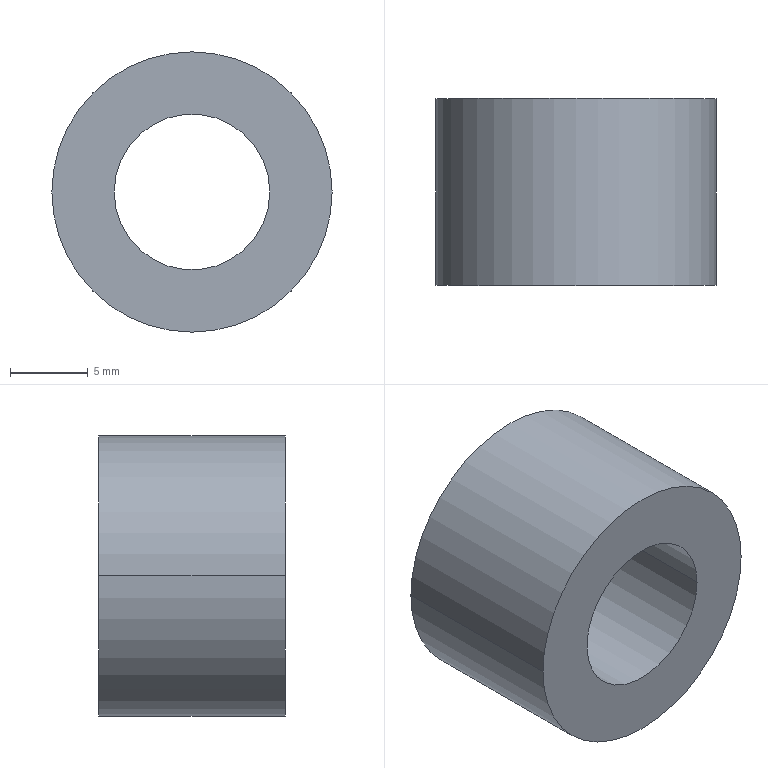Part | SolidWorks | features Revolution 1 | 1 solid | 6 faces | box 18 x 12 x 18 mm | volume 2111 mm3 | cylinder 4 | plane 2 | commonest cylinder face diameters 10 x2 18 x2
STEP:
#1=CARTESIAN_POINT('',(9.,12.,0.));
#2=VERTEX_POINT('',#1);
#3=CARTESIAN_POINT('',(-9.,12.,0.));
#4=VERTEX_POINT('',#3);
#5=CARTESIAN_POINT('',(0.,12.,0.));
#6=DIRECTION('',(0.,-1.,0.));
#7=DIRECTION('',(1.,0.,0.));
#8=AXIS2_PLACEMENT_3D('',#5,#6,#7);
#9=CIRCLE('',#8,9.);
#10=EDGE_CURVE('',#2,#4,#9,.T.);
#11=ORIENTED_EDGE('',*,*,#10,.T.);
#12=CARTESIAN_POINT('',(-9.,0.,0.));
#13=VERTEX_POINT('',#12);
#14=CARTESIAN_POINT('',(-9.,-483.484,0.));
#15=DIRECTION('',(0.,-1.,0.));
#16=VECTOR('',#15,1000.);
#17=LINE('',#14,#16);
#18=EDGE_CURVE('',#4,#13,#17,.T.);
#19=ORIENTED_EDGE('',*,*,#18,.T.);
#20=CARTESIAN_POINT('',(9.,0.,0.));
#21=VERTEX_POINT('',#20);
#22=CARTESIAN_POINT('',(0.,0.,0.));
#23=DIRECTION('',(0.,-1.,0.));
#24=DIRECTION('',(1.,0.,0.));
#25=AXIS2_PLACEMENT_3D('',#22,#23,#24);
#26=CIRCLE('',#25,9.);
#27=EDGE_CURVE('',#21,#13,#26,.T.);
#28=ORIENTED_EDGE('',*,*,#27,.F.);
#29=CARTESIAN_POINT('',(9.,-483.484,0.));
#30=DIRECTION('',(0.,-1.,0.));
#31=VECTOR('',#30,1000.);
#32=LINE('',#29,#31);
#33=EDGE_CURVE('',#2,#21,#32,.T.);
#34=ORIENTED_EDGE('',*,*,#33,.F.);
#35=EDGE_LOOP('',(#11,#19,#28,#34));
#36=FACE_OUTER_BOUND('',#35,.T.);
#37=CARTESIAN_POINT('',(0.,-483.484,0.));
#38=DIRECTION('',(0.,-1.,0.));
#39=DIRECTION('',(1.,0.,0.));
#40=AXIS2_PLACEMENT_3D('',#37,#38,#39);
#41=CYLINDRICAL_SURFACE('',#40,9.);
#42=ADVANCED_FACE('',(#36),#41,.T.);
#43=CARTESIAN_POINT('',(-5.,12.,0.));
#44=VERTEX_POINT('',#43);
#45=CARTESIAN_POINT('',(5.,12.,0.));
#46=VERTEX_POINT('',#45);
#47=CARTESIAN_POINT('',(0.,12.,0.));
#48=DIRECTION('',(0.,-1.,0.));
#49=DIRECTION('',(1.,0.,0.));
#50=AXIS2_PLACEMENT_3D('',#47,#48,#49);
#51=CIRCLE('',#50,5.);
#52=EDGE_CURVE('',#44,#46,#51,.T.);
#53=ORIENTED_EDGE('',*,*,#52,.F.);
#54=CARTESIAN_POINT('',(-5.,0.,0.));
#55=VERTEX_POINT('',#54);
#56=CARTESIAN_POINT('',(-5.,-483.484,0.));
#57=DIRECTION('',(0.,-1.,0.));
#58=VECTOR('',#57,1000.);
#59=LINE('',#56,#58);
#60=EDGE_CURVE('',#44,#55,#59,.T.);
#61=ORIENTED_EDGE('',*,*,#60,.T.);
#62=CARTESIAN_POINT('',(5.,0.,0.));
#63=VERTEX_POINT('',#62);
#64=CARTESIAN_POINT('',(0.,0.,0.));
#65=DIRECTION('',(0.,-1.,0.));
#66=DIRECTION('',(1.,0.,0.));
#67=AXIS2_PLACEMENT_3D('',#64,#65,#66);
#68=CIRCLE('',#67,5.);
#69=EDGE_CURVE('',#55,#63,#68,.T.);
#70=ORIENTED_EDGE('',*,*,#69,.T.);
#71=CARTESIAN_POINT('',(5.,-483.484,0.));
#72=DIRECTION('',(0.,-1.,0.));
#73=VECTOR('',#72,1000.);
#74=LINE('',#71,#73);
#75=EDGE_CURVE('',#46,#63,#74,.T.);
#76=ORIENTED_EDGE('',*,*,#75,.F.);
#77=EDGE_LOOP('',(#53,#61,#70,#76));
#78=FACE_OUTER_BOUND('',#77,.T.);
#79=CARTESIAN_POINT('',(0.,-483.484,0.));
#80=DIRECTION('',(0.,-1.,0.));
#81=DIRECTION('',(1.,0.,0.));
#82=AXIS2_PLACEMENT_3D('',#79,#80,#81);
#83=CYLINDRICAL_SURFACE('',#82,5.);
#84=ADVANCED_FACE('',(#78),#83,.F.);
#85=ORIENTED_EDGE('',*,*,#60,.F.);
#86=CARTESIAN_POINT('',(0.,12.,0.));
#87=DIRECTION('',(0.,-1.,0.));
#88=DIRECTION('',(1.,0.,0.));
#89=AXIS2_PLACEMENT_3D('',#86,#87,#88);
#90=CIRCLE('',#89,5.);
#91=EDGE_CURVE('',#46,#44,#90,.T.);
#92=ORIENTED_EDGE('',*,*,#91,.F.);
#93=ORIENTED_EDGE('',*,*,#75,.T.);
#94=CARTESIAN_POINT('',(0.,0.,0.));
#95=DIRECTION('',(0.,-1.,0.));
#96=DIRECTION('',(1.,0.,0.));
#97=AXIS2_PLACEMENT_3D('',#94,#95,#96);
#98=CIRCLE('',#97,5.);
#99=EDGE_CURVE('',#63,#55,#98,.T.);
#100=ORIENTED_EDGE('',*,*,#99,.T.);
#101=EDGE_LOOP('',(#85,#92,#93,#100));
#102=FACE_OUTER_BOUND('',#101,.T.);
#103=CARTESIAN_POINT('',(0.,-483.484,0.));
#104=DIRECTION('',(0.,-1.,0.));
#105=DIRECTION('',(1.,0.,0.));
#106=AXIS2_PLACEMENT_3D('',#103,#104,#105);
#107=CYLINDRICAL_SURFACE('',#106,5.);
#108=ADVANCED_FACE('',(#102),#107,.F.);
#109=ORIENTED_EDGE('',*,*,#27,.T.);
#110=CARTESIAN_POINT('',(0.,0.,0.));
#111=DIRECTION('',(0.,-1.,0.));
#112=DIRECTION('',(1.,0.,0.));
#113=AXIS2_PLACEMENT_3D('',#110,#111,#112);
#114=CIRCLE('',#113,9.);
#115=EDGE_CURVE('',#13,#21,#114,.T.);
#116=ORIENTED_EDGE('',*,*,#115,.T.);
#117=EDGE_LOOP('',(#109,#116));
#118=FACE_OUTER_BOUND('',#117,.T.);
#119=ORIENTED_EDGE('',*,*,#99,.F.);
#120=ORIENTED_EDGE('',*,*,#69,.F.);
#121=EDGE_LOOP('',(#119,#120));
#122=FACE_BOUND('',#121,.T.);
#123=CARTESIAN_POINT('',(5.,0.,0.));
#124=DIRECTION('',(0.,-1.,0.));
#125=DIRECTION('',(1.,0.,0.));
#126=AXIS2_PLACEMENT_3D('',#123,#124,#125);
#127=PLANE('',#126);
#128=ADVANCED_FACE('',(#118,#122),#127,.T.);
#129=ORIENTED_EDGE('',*,*,#18,.F.);
#130=CARTESIAN_POINT('',(0.,12.,0.));
#131=DIRECTION('',(0.,-1.,0.));
#132=DIRECTION('',(1.,0.,0.));
#133=AXIS2_PLACEMENT_3D('',#130,#131,#132);
#134=CIRCLE('',#133,9.);
#135=EDGE_CURVE('',#4,#2,#134,.T.);
#136=ORIENTED_EDGE('',*,*,#135,.T.);
#137=ORIENTED_EDGE('',*,*,#33,.T.);
#138=ORIENTED_EDGE('',*,*,#115,.F.);
#139=EDGE_LOOP('',(#129,#136,#137,#138));
#140=FACE_OUTER_BOUND('',#139,.T.);
#141=CARTESIAN_POINT('',(0.,-483.484,0.));
#142=DIRECTION('',(0.,-1.,0.));
#143=DIRECTION('',(1.,0.,0.));
#144=AXIS2_PLACEMENT_3D('',#141,#142,#143);
#145=CYLINDRICAL_SURFACE('',#144,9.);
#146=ADVANCED_FACE('',(#140),#145,.T.);
#147=ORIENTED_EDGE('',*,*,#91,.T.);
#148=ORIENTED_EDGE('',*,*,#52,.T.);
#149=EDGE_LOOP('',(#147,#148));
#150=FACE_BOUND('',#149,.T.);
#151=ORIENTED_EDGE('',*,*,#10,.F.);
#152=ORIENTED_EDGE('',*,*,#135,.F.);
#153=EDGE_LOOP('',(#151,#152));
#154=FACE_OUTER_BOUND('',#153,.T.);
#155=CARTESIAN_POINT('',(5.,12.,0.));
#156=DIRECTION('',(0.,1.,0.));
#157=DIRECTION('',(-1.,0.,0.));
#158=AXIS2_PLACEMENT_3D('',#155,#156,#157);
#159=PLANE('',#158);
#160=ADVANCED_FACE('',(#150,#154),#159,.T.);
#161=CLOSED_SHELL('',(#42,#84,#108,#128,#146,#160));
#162=MANIFOLD_SOLID_BREP('',#161);
#163=CARTESIAN_POINT('',(0.,0.,0.));
#164=DIRECTION('',(0.,0.,1.));
#165=DIRECTION('',(1.,0.,0.));
#166=AXIS2_PLACEMENT_3D('',#163,#164,#165);
#167=(LENGTH_UNIT()NAMED_UNIT(*)SI_UNIT(.MILLI.,.METRE.));
#168=UNCERTAINTY_MEASURE_WITH_UNIT(LENGTH_MEASURE(0.00001),#167,'','');
#169=(NAMED_UNIT(*)PLANE_ANGLE_UNIT()SI_UNIT($,.RADIAN.));
#170=(NAMED_UNIT(*)SI_UNIT($,.STERADIAN.)SOLID_ANGLE_UNIT());
#171=(GEOMETRIC_REPRESENTATION_CONTEXT(3)GLOBAL_UNCERTAINTY_ASSIGNED_CONTEXT((#168))GLOBAL_UNIT_ASSIGNED_CONTEXT((#167,#169,#170))REPRESENTATION_CONTEXT('',''));
#172=ADVANCED_BREP_SHAPE_REPRESENTATION('',(#162,#166),#171);